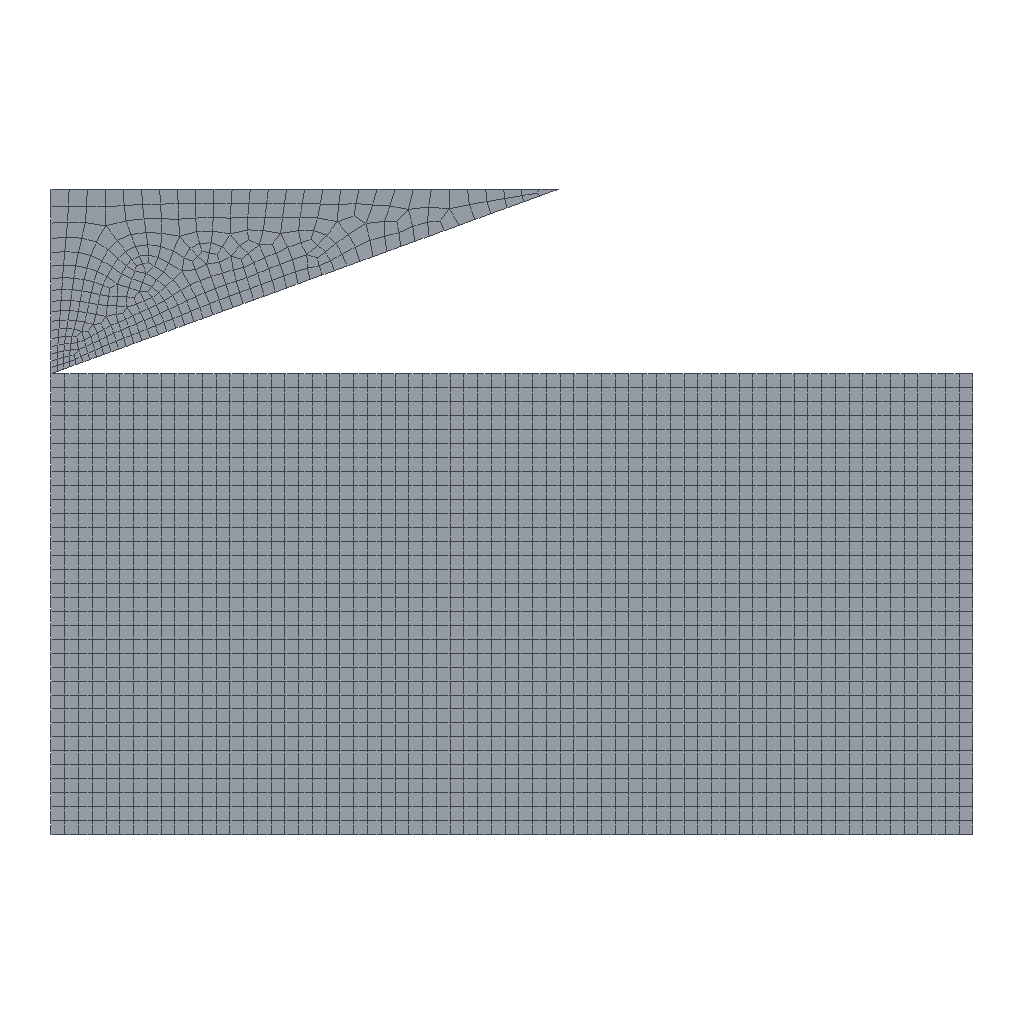Simulation study | abaqus
Set-up summary:
category,name,step,type,value,unit,region
solver,abaqus
solver,version,,,Abaqus/Standard 2020
units,not stated in the deck,,not stated
analysis,deck,,static,static
load_step,Step-1,Step-1,static
load_step,Step-2,Step-2,transient
load_step,requested,,,2
mesh,nodes,,,2688
mesh,elements,,,2540
element_type,CPE4,,plane,2211
element_type,CPS4R,,plane,329
load,load commands in deck,,count,1
bc,support commands in deck,,count,5
material,TOOL,,in results
material,WORK,,in results
check,setup vs results,,match,"per instance, exact: element labels, types and connectivity; labels of the nodes the elements use; coordinates of those nodes at SINGLE_PRECISION in 2 of 2 instance(s)"
Abaqus input file, long lists of numbers shortened:
*Heading
** Job name: Job-1 Model name: Model-1
** Generated by: Abaqus/CAE 2020
*Preprint, echo=NO, model=NO, history=NO, contact=NO
**
** PARTS
**
*Part, name=tou
*Node
      1,           0.,         -20.
      2,           0.,           0.
** (374 more lines like these left out)
*Element, type=CPS4R
  1, 321, 338, 339, 359
  2,   4,   1,  65,  93
** (327 more lines like these left out)
*Nset, nset=Set-1, generate
   1,  376,    1
*Elset, elset=Set-1, generate
   1,  329,    1
** Section: Section-2
*Solid Section, elset=Set-1, material=tool
,
*End Part
**
*Part, name=work
*Node
      1,         100.,           0.
      2,   98.507,           0.
** (2310 more lines like these left out)
*Element, type=CPE4
   1,    1,    2,   70,   69
   2,    2,    3,   71,   70
** (2209 more lines like these left out)
*Nset, nset=Set-1, generate
    1,  2312,     1
*Elset, elset=Set-1, generate
    1,  2211,     1
** Section: Section-1
*Solid Section, elset=Set-1, material=work
,
*End Part
**
**
** ASSEMBLY
**
*Assembly, name=Assembly
**
*Instance, name=tou-1, part=tou
          0.,          20.,           0.
*End Instance
**
*Instance, name=work-1, part=work
*End Instance
**
*Node
      1,           0.,          20.,           0.
*Nset, nset=Set-3, instance=work-1, generate
 2245,  2312,     1
*Elset, elset=Set-3, instance=work-1, generate
 2145,  2211,     1
*Nset, nset=Set-4
 1,
*Nset, nset=Set-5, instance=work-1, generate
   68,  2312,    68
*Elset, elset=Set-5, instance=work-1, generate
   67,  2211,    67
*Nset, nset=b_Set-1, instance=tou-1, generate
   1,  376,    1
*Elset, elset=b_Set-1, instance=tou-1, generate
   1,  329,    1
*Nset, nset=_PickedSet8, internal
 1,
*Elset, elset=_m_Surf-1_S1, internal, instance=tou-1
   2,   5,   6,   8,  11,  12,  13,  14,  15,  17,  18,  20,  55,  82,  83, 270
 298, 300, 302, 326
*Elset, elset=_m_Surf-1_S3, internal, instance=tou-1
  4, 23, 56, 76, 77, 80
*Elset, elset=_m_Surf-1_S2, internal, instance=tou-1
   2,   3,   9,  17,  22,  54,  79,  94, 112, 119, 120, 122, 279, 289, 295, 301
 312, 317, 321, 322, 323, 324, 325
*Elset, elset=_m_Surf-1_S4, internal, instance=tou-1
  19,  21,  24,  25,  26,  27,  28,  29,  30,  31,  32,  33,  34,  35,  36,  37
  38,  39,  40,  41,  42,  43,  44,  45,  46,  47,  48,  49,  50,  51,  55,  78
** (1 more lines like these left out)
*Surface, type=ELEMENT, name=m_Surf-1
_m_Surf-1_S1, S1
_m_Surf-1_S3, S3
_m_Surf-1_S2, S2
_m_Surf-1_S4, S4
*Elset, elset=_s_Surf-1_S1, internal, instance=work-1, generate
  1,  67,   1
*Elset, elset=_s_Surf-1_S2, internal, instance=work-1, generate
   67,  2211,    67
*Surface, type=ELEMENT, name=s_Surf-1
_s_Surf-1_S1, S1
_s_Surf-1_S2, S2
** Constraint: Constraint-1
*Rigid Body, ref node=_PickedSet8, elset=b_Set-1, position=CENTER OF MASS
*End Assembly
*Amplitude, name=Amp-1
             0.,              0.,              1.,              1.
**
** MATERIALS
**
*Material, name=tool
*Density
 7.8e-09,
*Elastic
210000., 0.3
*Material, name=work
*Creep
1., 0.8, 0.6
*Elastic
1000., 0.4
*Plastic
50.,0.
**
** INTERACTION PROPERTIES
**
*Surface Interaction, name=IntProp-1
1.,
*Friction, slip tolerance=0.005
 0.2,
*Surface Behavior, pressure-overclosure=HARD
**
** INTERACTIONS
**
** Interaction: Int-1
*Contact Pair, interaction=IntProp-1, type=SURFACE TO SURFACE
s_Surf-1, m_Surf-1
** ----------------------------------------------------------------
**
** STEP: Step-1
**
*Step, name=Step-1, nlgeom=YES
*Static, stabilize=0.0002, allsdtol=0.05, continue=NO
0.01, 1., 1e-05, 1.
**
** BOUNDARY CONDITIONS
**
** Name: BC-1 Type: 对称/反对称/完全固定
*Boundary
Set-3, ENCASTRE
** Name: BC-2 Type: 位移/转角
*Boundary, amplitude=Amp-1
Set-4, 1, 1
Set-4, 2, 2, -5.
Set-4, 6, 6
** Name: BC-3 Type: 对称/反对称/完全固定
*Boundary
Set-5, XSYMM
**
** OUTPUT REQUESTS
**
*Restart, write, frequency=0
**
** FIELD OUTPUT: F-Output-1
**
*Output, field
*Node Output
CF, RF, U, V
*Element Output, directions=YES
E, LE, MISES, MISESMAX, PE, PEEQ, PEEQT, S, VE, VEEQ, VS
*Contact Output
CDISP, CSTRESS
**
** HISTORY OUTPUT: H-Output-1
**
*Output, history, variable=PRESELECT
*End Step
** ----------------------------------------------------------------
**
** STEP: Step-2
**
*Step, name=Step-2, nlgeom=YES, inc=10000
*Visco, cetol=1.
0.0001, 50., 5e-06, 50.
**
** OUTPUT REQUESTS
**
*Restart, write, frequency=0
**
** FIELD OUTPUT: F-Output-1
**
*Output, field
*Node Output
CF, RF, U, V
*Element Output, directions=YES
CE, CEEQ, CEMAG, CEP, E, LE, MISES, MISESMAX, PE, PEEQ, PEEQT, S, VE, VEEQ, VS
*Contact Output
CDISP, CSTRESS
**
** HISTORY OUTPUT: H-Output-1
**
*Output, history, variable=PRESELECT
*End Step
Results summary:
result,step,,completed,increments=17 time=1.0/1.0
result,step,,partial,increments=508 time=0.05368/50.0
result,analysis,,,transient
result,last_loadstep,,,2
result,primary field,,,U
result,reaction total,,FX,-0.0,model units
result,reaction total,,FY,-0.0,model units
result,reaction total,,FZ,0.0,model units